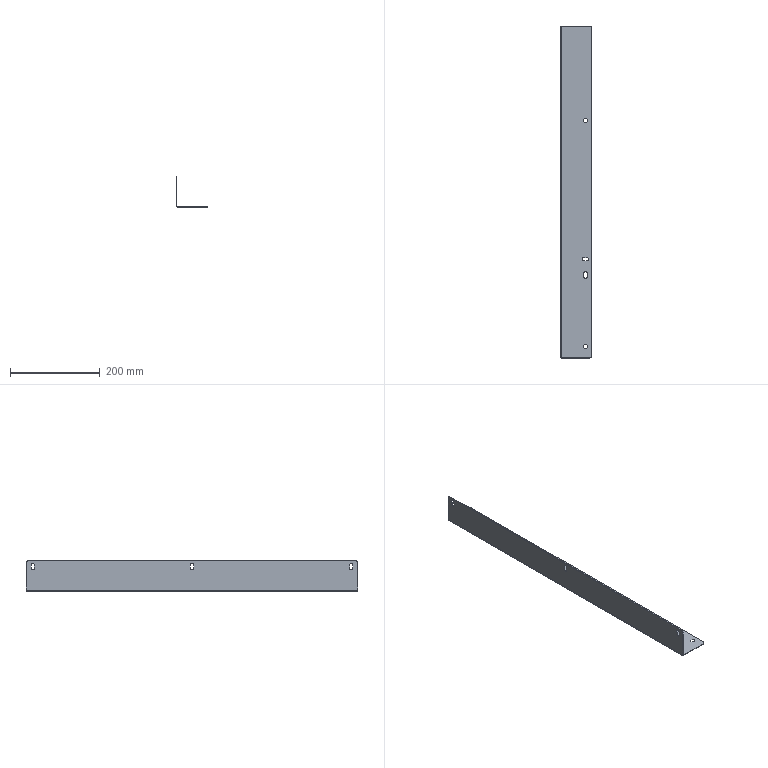Part | SolidWorks | features BaseBody 1 | 1 solid | 54 faces | box 70 x 740 x 67.2 mm | volume 119393 mm3 | plane 34 | cylinder 20 | commonest cylinder face diameters 7 x14 10 x4 2 x1 4.4 x1